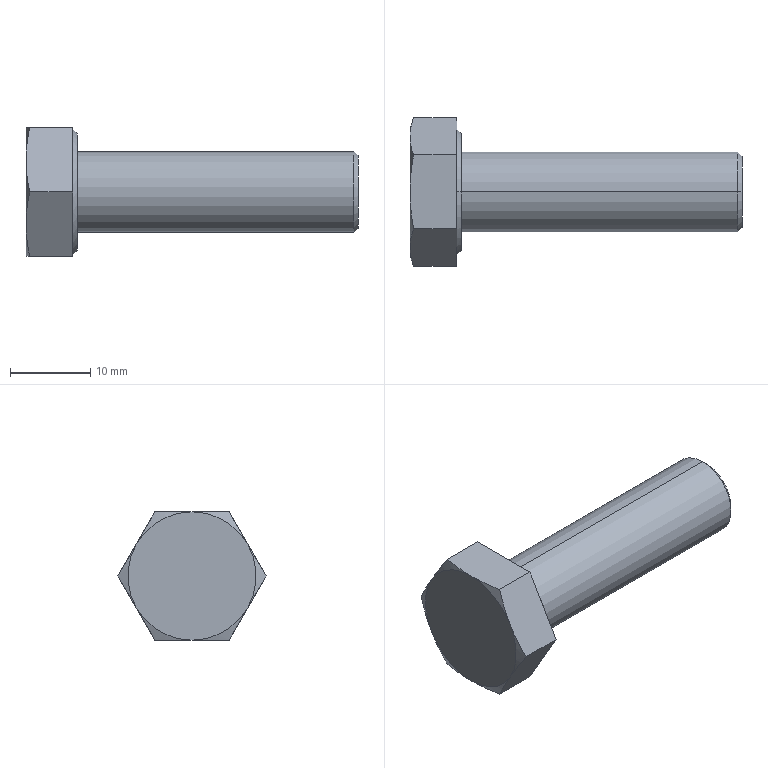Part | SolidWorks | features RevCut 3, Boss 1, Chamfer 1, Extrusion 1, Fillet 1, LPattern 1 | 1 solid | 22 faces | box 41.4 x 18.475 x 16 mm | volume 4135 mm3 | cone 10 | plane 10 | cylinder 2 | commonest cylinder face diameters 10 x2
STEP:
#1=CARTESIAN_POINT('',(41.4,0.,-4.5));
#2=VERTEX_POINT('',#1);
#3=CARTESIAN_POINT('',(41.4,0.,4.5));
#4=VERTEX_POINT('',#3);
#5=CARTESIAN_POINT('',(41.4,0.,0.));
#6=DIRECTION('',(1.,0.,0.));
#7=DIRECTION('',(0.,0.,-1.));
#8=AXIS2_PLACEMENT_3D('',#5,#6,#7);
#9=CIRCLE('',#8,4.5);
#10=EDGE_CURVE('',#2,#4,#9,.T.);
#11=ORIENTED_EDGE('',*,*,#10,.F.);
#12=CARTESIAN_POINT('',(40.9,0.,-5.));
#13=VERTEX_POINT('',#12);
#14=CARTESIAN_POINT('',(41.4,0.,-4.5));
#15=DIRECTION('',(-0.7071,0.,-0.7071));
#16=VECTOR('',#15,1000.);
#17=LINE('',#14,#16);
#18=EDGE_CURVE('',#2,#13,#17,.T.);
#19=ORIENTED_EDGE('',*,*,#18,.T.);
#20=CARTESIAN_POINT('',(40.9,0.,5.));
#21=VERTEX_POINT('',#20);
#22=CARTESIAN_POINT('',(40.9,0.,0.));
#23=DIRECTION('',(-1.,0.,0.));
#24=DIRECTION('',(0.,0.,-1.));
#25=AXIS2_PLACEMENT_3D('',#22,#23,#24);
#26=CIRCLE('',#25,5.);
#27=EDGE_CURVE('',#21,#13,#26,.T.);
#28=ORIENTED_EDGE('',*,*,#27,.F.);
#29=CARTESIAN_POINT('',(41.4,0.,4.5));
#30=DIRECTION('',(-0.7071,0.,0.7071));
#31=VECTOR('',#30,1000.);
#32=LINE('',#29,#31);
#33=EDGE_CURVE('',#4,#21,#32,.T.);
#34=ORIENTED_EDGE('',*,*,#33,.F.);
#35=EDGE_LOOP('',(#11,#19,#28,#34));
#36=FACE_OUTER_BOUND('',#35,.T.);
#37=CARTESIAN_POINT('',(41.4,0.,0.));
#38=DIRECTION('',(-1.,0.,0.));
#39=DIRECTION('',(0.,0.,1.));
#40=AXIS2_PLACEMENT_3D('',#37,#38,#39);
#41=CONICAL_SURFACE('',#40,4.5,0.7854);
#42=ADVANCED_FACE('',(#36),#41,.T.);
#43=ORIENTED_EDGE('',*,*,#27,.T.);
#44=CARTESIAN_POINT('',(6.4,0.,-5.));
#45=VERTEX_POINT('',#44);
#46=CARTESIAN_POINT('',(41.4,0.,-5.));
#47=DIRECTION('',(-1.,0.,0.));
#48=VECTOR('',#47,1000.);
#49=LINE('',#46,#48);
#50=EDGE_CURVE('',#13,#45,#49,.T.);
#51=ORIENTED_EDGE('',*,*,#50,.T.);
#52=CARTESIAN_POINT('',(6.4,0.,5.));
#53=VERTEX_POINT('',#52);
#54=CARTESIAN_POINT('',(6.4,0.,0.));
#55=DIRECTION('',(1.,0.,0.));
#56=DIRECTION('',(0.,0.,1.));
#57=AXIS2_PLACEMENT_3D('',#54,#55,#56);
#58=CIRCLE('',#57,5.);
#59=EDGE_CURVE('',#45,#53,#58,.T.);
#60=ORIENTED_EDGE('',*,*,#59,.T.);
#61=CARTESIAN_POINT('',(41.4,0.,5.));
#62=DIRECTION('',(-1.,0.,0.));
#63=VECTOR('',#62,1000.);
#64=LINE('',#61,#63);
#65=EDGE_CURVE('',#21,#53,#64,.T.);
#66=ORIENTED_EDGE('',*,*,#65,.F.);
#67=EDGE_LOOP('',(#43,#51,#60,#66));
#68=FACE_OUTER_BOUND('',#67,.T.);
#69=CARTESIAN_POINT('',(41.4,0.,0.));
#70=DIRECTION('',(-1.,0.,0.));
#71=DIRECTION('',(0.,0.,1.));
#72=AXIS2_PLACEMENT_3D('',#69,#70,#71);
#73=CYLINDRICAL_SURFACE('',#72,5.);
#74=ADVANCED_FACE('',(#68),#73,.T.);
#75=CARTESIAN_POINT('',(6.4,0.,7.235));
#76=VERTEX_POINT('',#75);
#77=CARTESIAN_POINT('',(6.4,0.,-7.235));
#78=VERTEX_POINT('',#77);
#79=CARTESIAN_POINT('',(6.4,0.,0.));
#80=DIRECTION('',(-1.,0.,0.));
#81=DIRECTION('',(0.,0.,1.));
#82=AXIS2_PLACEMENT_3D('',#79,#80,#81);
#83=CIRCLE('',#82,7.235);
#84=EDGE_CURVE('',#76,#78,#83,.T.);
#85=ORIENTED_EDGE('',*,*,#84,.T.);
#86=CARTESIAN_POINT('',(5.8,0.,-7.835));
#87=VERTEX_POINT('',#86);
#88=CARTESIAN_POINT('',(5.8,0.,-7.835));
#89=DIRECTION('',(-0.7071,0.,-0.7071));
#90=VECTOR('',#89,1000.);
#91=LINE('',#88,#90);
#92=EDGE_CURVE('',#78,#87,#91,.T.);
#93=ORIENTED_EDGE('',*,*,#92,.T.);
#94=CARTESIAN_POINT('',(5.8,0.,7.835));
#95=VERTEX_POINT('',#94);
#96=CARTESIAN_POINT('',(5.8,0.,0.));
#97=DIRECTION('',(-1.,0.,0.));
#98=DIRECTION('',(0.,0.,1.));
#99=AXIS2_PLACEMENT_3D('',#96,#97,#98);
#100=CIRCLE('',#99,7.835);
#101=EDGE_CURVE('',#95,#87,#100,.T.);
#102=ORIENTED_EDGE('',*,*,#101,.F.);
#103=CARTESIAN_POINT('',(5.8,0.,7.835));
#104=DIRECTION('',(-0.7071,0.,0.7071));
#105=VECTOR('',#104,1000.);
#106=LINE('',#103,#105);
#107=EDGE_CURVE('',#76,#95,#106,.T.);
#108=ORIENTED_EDGE('',*,*,#107,.F.);
#109=EDGE_LOOP('',(#85,#93,#102,#108));
#110=FACE_OUTER_BOUND('',#109,.T.);
#111=CARTESIAN_POINT('',(5.8,0.,0.));
#112=DIRECTION('',(-1.,0.,0.));
#113=DIRECTION('',(0.,0.,1.));
#114=AXIS2_PLACEMENT_3D('',#111,#112,#113);
#115=CONICAL_SURFACE('',#114,7.835,0.7854);
#116=ADVANCED_FACE('',(#110),#115,.T.);
#117=ORIENTED_EDGE('',*,*,#84,.F.);
#118=CARTESIAN_POINT('',(6.4,0.,0.));
#119=DIRECTION('',(-1.,0.,0.));
#120=DIRECTION('',(0.,0.,1.));
#121=AXIS2_PLACEMENT_3D('',#118,#119,#120);
#122=CIRCLE('',#121,7.235);
#123=EDGE_CURVE('',#78,#76,#122,.T.);
#124=ORIENTED_EDGE('',*,*,#123,.F.);
#125=EDGE_LOOP('',(#117,#124));
#126=FACE_OUTER_BOUND('',#125,.T.);
#127=CARTESIAN_POINT('',(6.4,0.,0.));
#128=DIRECTION('',(1.,0.,0.));
#129=DIRECTION('',(0.,0.,1.));
#130=AXIS2_PLACEMENT_3D('',#127,#128,#129);
#131=CIRCLE('',#130,5.);
#132=EDGE_CURVE('',#53,#45,#131,.T.);
#133=ORIENTED_EDGE('',*,*,#132,.F.);
#134=ORIENTED_EDGE('',*,*,#59,.F.);
#135=EDGE_LOOP('',(#133,#134));
#136=FACE_BOUND('',#135,.T.);
#137=CARTESIAN_POINT('',(6.4,0.,16.));
#138=DIRECTION('',(-1.,0.,0.));
#139=DIRECTION('',(0.,0.,1.));
#140=AXIS2_PLACEMENT_3D('',#137,#138,#139);
#141=PLANE('',#140);
#142=ADVANCED_FACE('',(#126,#136),#141,.F.);
#143=CARTESIAN_POINT('',(0.4505,-9.238,0.));
#144=VERTEX_POINT('',#143);
#145=CARTESIAN_POINT('',(0.,-6.928,4.));
#146=VERTEX_POINT('',#145);
#147=CARTESIAN_POINT('',(0.4505,-9.238,0.));
#148=CARTESIAN_POINT('',(0.3104,-8.853,0.6667));
#149=CARTESIAN_POINT('',(0.1966,-8.468,1.333));
#150=CARTESIAN_POINT('',(0.04119,-7.698,2.667));
#151=CARTESIAN_POINT('',(0.,-7.313,3.333));
#152=CARTESIAN_POINT('',(0.,-6.928,4.));
#153=B_SPLINE_CURVE_WITH_KNOTS('',3,(#147,#148,#149,#150,#151,#152),.UNSPECIFIED.,.F.,.F.,(4,2,4),(0.000000231,0.00231,0.004619),.UNSPECIFIED.);
#154=EDGE_CURVE('',#144,#146,#153,.T.);
#155=ORIENTED_EDGE('',*,*,#154,.F.);
#156=CARTESIAN_POINT('',(5.8,-9.238,0.));
#157=VERTEX_POINT('',#156);
#158=CARTESIAN_POINT('',(6.4,-9.238,0.));
#159=DIRECTION('',(-1.,0.,0.));
#160=VECTOR('',#159,1000.);
#161=LINE('',#158,#160);
#162=EDGE_CURVE('',#157,#144,#161,.T.);
#163=ORIENTED_EDGE('',*,*,#162,.F.);
#164=CARTESIAN_POINT('',(5.8,-4.619,8.));
#165=VERTEX_POINT('',#164);
#166=CARTESIAN_POINT('',(5.8,-4.619,8.));
#167=DIRECTION('',(0.,-0.5,-0.866));
#168=VECTOR('',#167,1000.);
#169=LINE('',#166,#168);
#170=EDGE_CURVE('',#165,#157,#169,.T.);
#171=ORIENTED_EDGE('',*,*,#170,.F.);
#172=CARTESIAN_POINT('',(0.4505,-4.619,8.));
#173=VERTEX_POINT('',#172);
#174=CARTESIAN_POINT('',(6.4,-4.619,8.));
#175=DIRECTION('',(-1.,0.,0.));
#176=VECTOR('',#175,1000.);
#177=LINE('',#174,#176);
#178=EDGE_CURVE('',#165,#173,#177,.T.);
#179=ORIENTED_EDGE('',*,*,#178,.T.);
#180=CARTESIAN_POINT('',(0.,-6.928,4.));
#181=CARTESIAN_POINT('',(0.,-6.543,4.667));
#182=CARTESIAN_POINT('',(0.04119,-6.158,5.333));
#183=CARTESIAN_POINT('',(0.1966,-5.389,6.667));
#184=CARTESIAN_POINT('',(0.3104,-5.004,7.333));
#185=CARTESIAN_POINT('',(0.4505,-4.619,8.));
#186=B_SPLINE_CURVE_WITH_KNOTS('',3,(#180,#181,#182,#183,#184,#185),.UNSPECIFIED.,.F.,.F.,(4,2,4),(0.004619,0.006928,0.009238),.UNSPECIFIED.);
#187=EDGE_CURVE('',#146,#173,#186,.T.);
#188=ORIENTED_EDGE('',*,*,#187,.F.);
#189=EDGE_LOOP('',(#155,#163,#171,#179,#188));
#190=FACE_OUTER_BOUND('',#189,.T.);
#191=CARTESIAN_POINT('',(6.4,-4.619,8.));
#192=DIRECTION('',(0.,0.866,-0.5));
#193=DIRECTION('',(0.,0.5,0.866));
#194=AXIS2_PLACEMENT_3D('',#191,#192,#193);
#195=PLANE('',#194);
#196=ADVANCED_FACE('',(#190),#195,.F.);
#197=CARTESIAN_POINT('',(0.4505,-4.619,-8.));
#198=VERTEX_POINT('',#197);
#199=CARTESIAN_POINT('',(0.,-6.928,-4.));
#200=VERTEX_POINT('',#199);
#201=CARTESIAN_POINT('',(0.4505,-4.619,-8.));
#202=CARTESIAN_POINT('',(0.3104,-5.004,-7.333));
#203=CARTESIAN_POINT('',(0.1966,-5.389,-6.667));
#204=CARTESIAN_POINT('',(0.04119,-6.158,-5.333));
#205=CARTESIAN_POINT('',(0.,-6.543,-4.667));
#206=CARTESIAN_POINT('',(0.,-6.928,-4.));
#207=B_SPLINE_CURVE_WITH_KNOTS('',3,(#201,#202,#203,#204,#205,#206),.UNSPECIFIED.,.F.,.F.,(4,2,4),(0.000000231,0.00231,0.004619),.UNSPECIFIED.);
#208=EDGE_CURVE('',#198,#200,#207,.T.);
#209=ORIENTED_EDGE('',*,*,#208,.F.);
#210=CARTESIAN_POINT('',(5.8,-4.619,-8.));
#211=VERTEX_POINT('',#210);
#212=CARTESIAN_POINT('',(6.4,-4.619,-8.));
#213=DIRECTION('',(-1.,0.,0.));
#214=VECTOR('',#213,1000.);
#215=LINE('',#212,#214);
#216=EDGE_CURVE('',#211,#198,#215,.T.);
#217=ORIENTED_EDGE('',*,*,#216,.F.);
#218=CARTESIAN_POINT('',(5.8,-9.238,0.));
#219=DIRECTION('',(0.,0.5,-0.866));
#220=VECTOR('',#219,1000.);
#221=LINE('',#218,#220);
#222=EDGE_CURVE('',#157,#211,#221,.T.);
#223=ORIENTED_EDGE('',*,*,#222,.F.);
#224=ORIENTED_EDGE('',*,*,#162,.T.);
#225=CARTESIAN_POINT('',(0.,-6.928,-4.));
#226=CARTESIAN_POINT('',(0.,-7.313,-3.333));
#227=CARTESIAN_POINT('',(0.04119,-7.698,-2.667));
#228=CARTESIAN_POINT('',(0.1966,-8.468,-1.333));
#229=CARTESIAN_POINT('',(0.3104,-8.853,-0.6667));
#230=CARTESIAN_POINT('',(0.4505,-9.238,0.));
#231=B_SPLINE_CURVE_WITH_KNOTS('',3,(#225,#226,#227,#228,#229,#230),.UNSPECIFIED.,.F.,.F.,(4,2,4),(0.004619,0.006928,0.009238),.UNSPECIFIED.);
#232=EDGE_CURVE('',#200,#144,#231,.T.);
#233=ORIENTED_EDGE('',*,*,#232,.F.);
#234=EDGE_LOOP('',(#209,#217,#223,#224,#233));
#235=FACE_OUTER_BOUND('',#234,.T.);
#236=CARTESIAN_POINT('',(6.4,-9.238,0.));
#237=DIRECTION('',(0.,0.866,0.5));
#238=DIRECTION('',(0.,-0.5,0.866));
#239=AXIS2_PLACEMENT_3D('',#236,#237,#238);
#240=PLANE('',#239);
#241=ADVANCED_FACE('',(#235),#240,.F.);
#242=CARTESIAN_POINT('',(0.4505,4.619,-8.));
#243=VERTEX_POINT('',#242);
#244=CARTESIAN_POINT('',(0.,0.,-8.));
#245=VERTEX_POINT('',#244);
#246=CARTESIAN_POINT('',(0.4505,4.619,-8.));
#247=CARTESIAN_POINT('',(0.3107,3.851,-8.));
#248=CARTESIAN_POINT('',(0.1969,3.081,-8.));
#249=CARTESIAN_POINT('',(0.04135,1.542,-8.));
#250=CARTESIAN_POINT('',(0.,0.7714,-8.));
#251=CARTESIAN_POINT('',(0.,0.,-8.));
#252=B_SPLINE_CURVE_WITH_KNOTS('',3,(#246,#247,#248,#249,#250,#251),.UNSPECIFIED.,.F.,.F.,(4,2,4),(0.01666,0.01898,0.02131),.UNSPECIFIED.);
#253=EDGE_CURVE('',#243,#245,#252,.T.);
#254=ORIENTED_EDGE('',*,*,#253,.F.);
#255=CARTESIAN_POINT('',(5.8,4.619,-8.));
#256=VERTEX_POINT('',#255);
#257=CARTESIAN_POINT('',(6.4,4.619,-8.));
#258=DIRECTION('',(-1.,0.,0.));
#259=VECTOR('',#258,1000.);
#260=LINE('',#257,#259);
#261=EDGE_CURVE('',#256,#243,#260,.T.);
#262=ORIENTED_EDGE('',*,*,#261,.F.);
#263=CARTESIAN_POINT('',(5.8,-4.619,-8.));
#264=DIRECTION('',(0.,1.,0.));
#265=VECTOR('',#264,1000.);
#266=LINE('',#263,#265);
#267=EDGE_CURVE('',#211,#256,#266,.T.);
#268=ORIENTED_EDGE('',*,*,#267,.F.);
#269=ORIENTED_EDGE('',*,*,#216,.T.);
#270=CARTESIAN_POINT('',(0.,0.,-8.));
#271=CARTESIAN_POINT('',(0.,-0.7692,-8.));
#272=CARTESIAN_POINT('',(0.04113,-1.539,-8.));
#273=CARTESIAN_POINT('',(0.1968,-3.081,-8.));
#274=CARTESIAN_POINT('',(0.3113,-3.854,-8.));
#275=CARTESIAN_POINT('',(0.4505,-4.619,-8.));
#276=B_SPLINE_CURVE_WITH_KNOTS('',3,(#270,#271,#272,#273,#274,#275),.UNSPECIFIED.,.F.,.F.,(4,2,4),(0.02131,0.02363,0.02596),.UNSPECIFIED.);
#277=EDGE_CURVE('',#245,#198,#276,.T.);
#278=ORIENTED_EDGE('',*,*,#277,.F.);
#279=EDGE_LOOP('',(#254,#262,#268,#269,#278));
#280=FACE_OUTER_BOUND('',#279,.T.);
#281=CARTESIAN_POINT('',(6.4,-4.619,-8.));
#282=DIRECTION('',(0.,0.,1.));
#283=DIRECTION('',(0.,-1.,0.));
#284=AXIS2_PLACEMENT_3D('',#281,#282,#283);
#285=PLANE('',#284);
#286=ADVANCED_FACE('',(#280),#285,.F.);
#287=CARTESIAN_POINT('',(0.4505,9.238,0.));
#288=VERTEX_POINT('',#287);
#289=CARTESIAN_POINT('',(0.,6.928,-4.));
#290=VERTEX_POINT('',#289);
#291=CARTESIAN_POINT('',(0.4505,9.238,0.));
#292=CARTESIAN_POINT('',(0.3104,8.853,-0.6667));
#293=CARTESIAN_POINT('',(0.1966,8.468,-1.333));
#294=CARTESIAN_POINT('',(0.04119,7.698,-2.667));
#295=CARTESIAN_POINT('',(0.,7.313,-3.333));
#296=CARTESIAN_POINT('',(0.,6.928,-4.));
#297=B_SPLINE_CURVE_WITH_KNOTS('',3,(#291,#292,#293,#294,#295,#296),.UNSPECIFIED.,.F.,.F.,(4,2,4),(0.000000231,0.00231,0.004619),.UNSPECIFIED.);
#298=EDGE_CURVE('',#288,#290,#297,.T.);
#299=ORIENTED_EDGE('',*,*,#298,.F.);
#300=CARTESIAN_POINT('',(5.8,9.238,0.));
#301=VERTEX_POINT('',#300);
#302=CARTESIAN_POINT('',(6.4,9.238,0.));
#303=DIRECTION('',(-1.,0.,0.));
#304=VECTOR('',#303,1000.);
#305=LINE('',#302,#304);
#306=EDGE_CURVE('',#301,#288,#305,.T.);
#307=ORIENTED_EDGE('',*,*,#306,.F.);
#308=CARTESIAN_POINT('',(5.8,4.619,-8.));
#309=DIRECTION('',(0.,0.5,0.866));
#310=VECTOR('',#309,1000.);
#311=LINE('',#308,#310);
#312=EDGE_CURVE('',#256,#301,#311,.T.);
#313=ORIENTED_EDGE('',*,*,#312,.F.);
#314=ORIENTED_EDGE('',*,*,#261,.T.);
#315=CARTESIAN_POINT('',(0.,6.928,-4.));
#316=CARTESIAN_POINT('',(0.,6.543,-4.667));
#317=CARTESIAN_POINT('',(0.04119,6.158,-5.333));
#318=CARTESIAN_POINT('',(0.1966,5.389,-6.667));
#319=CARTESIAN_POINT('',(0.3104,5.004,-7.333));
#320=CARTESIAN_POINT('',(0.4505,4.619,-8.));
#321=B_SPLINE_CURVE_WITH_KNOTS('',3,(#315,#316,#317,#318,#319,#320),.UNSPECIFIED.,.F.,.F.,(4,2,4),(0.004619,0.006928,0.009238),.UNSPECIFIED.);
#322=EDGE_CURVE('',#290,#243,#321,.T.);
#323=ORIENTED_EDGE('',*,*,#322,.F.);
#324=EDGE_LOOP('',(#299,#307,#313,#314,#323));
#325=FACE_OUTER_BOUND('',#324,.T.);
#326=CARTESIAN_POINT('',(6.4,4.619,-8.));
#327=DIRECTION('',(0.,-0.866,0.5));
#328=DIRECTION('',(0.,-0.5,-0.866));
#329=AXIS2_PLACEMENT_3D('',#326,#327,#328);
#330=PLANE('',#329);
#331=ADVANCED_FACE('',(#325),#330,.F.);
#332=CARTESIAN_POINT('',(0.4505,4.619,8.));
#333=VERTEX_POINT('',#332);
#334=CARTESIAN_POINT('',(0.,6.928,4.));
#335=VERTEX_POINT('',#334);
#336=CARTESIAN_POINT('',(0.4505,4.619,8.));
#337=CARTESIAN_POINT('',(0.3104,5.004,7.333));
#338=CARTESIAN_POINT('',(0.1966,5.389,6.667));
#339=CARTESIAN_POINT('',(0.04119,6.158,5.333));
#340=CARTESIAN_POINT('',(0.,6.543,4.667));
#341=CARTESIAN_POINT('',(0.,6.928,4.));
#342=B_SPLINE_CURVE_WITH_KNOTS('',3,(#336,#337,#338,#339,#340,#341),.UNSPECIFIED.,.F.,.F.,(4,2,4),(0.000000231,0.00231,0.004619),.UNSPECIFIED.);
#343=EDGE_CURVE('',#333,#335,#342,.T.);
#344=ORIENTED_EDGE('',*,*,#343,.F.);
#345=CARTESIAN_POINT('',(5.8,4.619,8.));
#346=VERTEX_POINT('',#345);
#347=CARTESIAN_POINT('',(6.4,4.619,8.));
#348=DIRECTION('',(-1.,0.,0.));
#349=VECTOR('',#348,1000.);
#350=LINE('',#347,#349);
#351=EDGE_CURVE('',#346,#333,#350,.T.);
#352=ORIENTED_EDGE('',*,*,#351,.F.);
#353=CARTESIAN_POINT('',(5.8,9.238,0.));
#354=DIRECTION('',(0.,-0.5,0.866));
#355=VECTOR('',#354,1000.);
#356=LINE('',#353,#355);
#357=EDGE_CURVE('',#301,#346,#356,.T.);
#358=ORIENTED_EDGE('',*,*,#357,.F.);
#359=ORIENTED_EDGE('',*,*,#306,.T.);
#360=CARTESIAN_POINT('',(0.,6.928,4.));
#361=CARTESIAN_POINT('',(0.,7.313,3.333));
#362=CARTESIAN_POINT('',(0.04119,7.698,2.667));
#363=CARTESIAN_POINT('',(0.1966,8.468,1.333));
#364=CARTESIAN_POINT('',(0.3104,8.853,0.6667));
#365=CARTESIAN_POINT('',(0.4505,9.238,0.));
#366=B_SPLINE_CURVE_WITH_KNOTS('',3,(#360,#361,#362,#363,#364,#365),.UNSPECIFIED.,.F.,.F.,(4,2,4),(0.004619,0.006928,0.009238),.UNSPECIFIED.);
#367=EDGE_CURVE('',#335,#288,#366,.T.);
#368=ORIENTED_EDGE('',*,*,#367,.F.);
#369=EDGE_LOOP('',(#344,#352,#358,#359,#368));
#370=FACE_OUTER_BOUND('',#369,.T.);
#371=CARTESIAN_POINT('',(6.4,9.238,0.));
#372=DIRECTION('',(0.,-0.866,-0.5));
#373=DIRECTION('',(0.,0.5,-0.866));
#374=AXIS2_PLACEMENT_3D('',#371,#372,#373);
#375=PLANE('',#374);
#376=ADVANCED_FACE('',(#370),#375,.F.);
#377=CARTESIAN_POINT('',(0.,0.,8.));
#378=VERTEX_POINT('',#377);
#379=CARTESIAN_POINT('',(0.4505,-4.619,8.));
#380=CARTESIAN_POINT('',(0.3113,-3.854,8.));
#381=CARTESIAN_POINT('',(0.1968,-3.081,8.));
#382=CARTESIAN_POINT('',(0.04113,-1.539,8.));
#383=CARTESIAN_POINT('',(0.,-0.7692,8.));
#384=CARTESIAN_POINT('',(0.,0.,8.));
#385=B_SPLINE_CURVE_WITH_KNOTS('',3,(#379,#380,#381,#382,#383,#384),.UNSPECIFIED.,.F.,.F.,(4,2,4),(0.007857,0.01018,0.01251),.UNSPECIFIED.);
#386=EDGE_CURVE('',#173,#378,#385,.T.);
#387=ORIENTED_EDGE('',*,*,#386,.F.);
#388=ORIENTED_EDGE('',*,*,#178,.F.);
#389=CARTESIAN_POINT('',(5.8,4.619,8.));
#390=DIRECTION('',(0.,-1.,0.));
#391=VECTOR('',#390,1000.);
#392=LINE('',#389,#391);
#393=EDGE_CURVE('',#346,#165,#392,.T.);
#394=ORIENTED_EDGE('',*,*,#393,.F.);
#395=ORIENTED_EDGE('',*,*,#351,.T.);
#396=CARTESIAN_POINT('',(0.,0.,8.));
#397=CARTESIAN_POINT('',(0.,0.7714,8.));
#398=CARTESIAN_POINT('',(0.04135,1.542,8.));
#399=CARTESIAN_POINT('',(0.1969,3.081,8.));
#400=CARTESIAN_POINT('',(0.3107,3.851,8.));
#401=CARTESIAN_POINT('',(0.4505,4.619,8.));
#402=B_SPLINE_CURVE_WITH_KNOTS('',3,(#396,#397,#398,#399,#400,#401),.UNSPECIFIED.,.F.,.F.,(4,2,4),(0.01251,0.01485,0.01718),.UNSPECIFIED.);
#403=EDGE_CURVE('',#378,#333,#402,.T.);
#404=ORIENTED_EDGE('',*,*,#403,.F.);
#405=EDGE_LOOP('',(#387,#388,#394,#395,#404));
#406=FACE_OUTER_BOUND('',#405,.T.);
#407=CARTESIAN_POINT('',(6.4,4.619,8.));
#408=DIRECTION('',(0.,0.,-1.));
#409=DIRECTION('',(-1.,0.,0.));
#410=AXIS2_PLACEMENT_3D('',#407,#408,#409);
#411=PLANE('',#410);
#412=ADVANCED_FACE('',(#406),#411,.F.);
#413=ORIENTED_EDGE('',*,*,#101,.T.);
#414=CARTESIAN_POINT('',(5.8,0.,0.));
#415=DIRECTION('',(-1.,0.,0.));
#416=DIRECTION('',(0.,0.,1.));
#417=AXIS2_PLACEMENT_3D('',#414,#415,#416);
#418=CIRCLE('',#417,7.835);
#419=EDGE_CURVE('',#87,#95,#418,.T.);
#420=ORIENTED_EDGE('',*,*,#419,.T.);
#421=EDGE_LOOP('',(#413,#420));
#422=FACE_BOUND('',#421,.T.);
#423=ORIENTED_EDGE('',*,*,#170,.T.);
#424=ORIENTED_EDGE('',*,*,#222,.T.);
#425=ORIENTED_EDGE('',*,*,#267,.T.);
#426=ORIENTED_EDGE('',*,*,#312,.T.);
#427=ORIENTED_EDGE('',*,*,#357,.T.);
#428=ORIENTED_EDGE('',*,*,#393,.T.);
#429=EDGE_LOOP('',(#423,#424,#425,#426,#427,#428));
#430=FACE_OUTER_BOUND('',#429,.T.);
#431=CARTESIAN_POINT('',(5.8,7.835,0.));
#432=DIRECTION('',(1.,0.,0.));
#433=DIRECTION('',(0.,0.,-1.));
#434=AXIS2_PLACEMENT_3D('',#431,#432,#433);
#435=PLANE('',#434);
#436=ADVANCED_FACE('',(#422,#430),#435,.T.);
#437=ORIENTED_EDGE('',*,*,#92,.F.);
#438=ORIENTED_EDGE('',*,*,#123,.T.);
#439=ORIENTED_EDGE('',*,*,#107,.T.);
#440=ORIENTED_EDGE('',*,*,#419,.F.);
#441=EDGE_LOOP('',(#437,#438,#439,#440));
#442=FACE_OUTER_BOUND('',#441,.T.);
#443=CARTESIAN_POINT('',(5.8,0.,0.));
#444=DIRECTION('',(-1.,0.,0.));
#445=DIRECTION('',(0.,0.,1.));
#446=AXIS2_PLACEMENT_3D('',#443,#444,#445);
#447=CONICAL_SURFACE('',#446,7.835,0.7854);
#448=ADVANCED_FACE('',(#442),#447,.T.);
#449=ORIENTED_EDGE('',*,*,#187,.T.);
#450=ORIENTED_EDGE('',*,*,#386,.T.);
#451=CARTESIAN_POINT('',(0.,0.,0.));
#452=DIRECTION('',(-1.,0.,0.));
#453=DIRECTION('',(0.,0.,1.));
#454=AXIS2_PLACEMENT_3D('',#451,#452,#453);
#455=CIRCLE('',#454,8.);
#456=EDGE_CURVE('',#146,#378,#455,.T.);
#457=ORIENTED_EDGE('',*,*,#456,.F.);
#458=EDGE_LOOP('',(#449,#450,#457));
#459=FACE_OUTER_BOUND('',#458,.T.);
#460=CARTESIAN_POINT('',(0.,0.,0.));
#461=DIRECTION('',(1.,0.,0.));
#462=DIRECTION('',(0.,0.,-1.));
#463=AXIS2_PLACEMENT_3D('',#460,#461,#462);
#464=CONICAL_SURFACE('',#463,8.,1.222);
#465=ADVANCED_FACE('',(#459),#464,.T.);
#466=ORIENTED_EDGE('',*,*,#232,.T.);
#467=ORIENTED_EDGE('',*,*,#154,.T.);
#468=CARTESIAN_POINT('',(0.,0.,0.));
#469=DIRECTION('',(-1.,0.,0.));
#470=DIRECTION('',(0.,0.,1.));
#471=AXIS2_PLACEMENT_3D('',#468,#469,#470);
#472=CIRCLE('',#471,8.);
#473=EDGE_CURVE('',#200,#146,#472,.T.);
#474=ORIENTED_EDGE('',*,*,#473,.F.);
#475=EDGE_LOOP('',(#466,#467,#474));
#476=FACE_OUTER_BOUND('',#475,.T.);
#477=CARTESIAN_POINT('',(0.,0.,0.));
#478=DIRECTION('',(1.,0.,0.));
#479=DIRECTION('',(0.,0.,-1.));
#480=AXIS2_PLACEMENT_3D('',#477,#478,#479);
#481=CONICAL_SURFACE('',#480,8.,1.222);
#482=ADVANCED_FACE('',(#476),#481,.T.);
#483=ORIENTED_EDGE('',*,*,#277,.T.);
#484=ORIENTED_EDGE('',*,*,#208,.T.);
#485=CARTESIAN_POINT('',(0.,0.,0.));
#486=DIRECTION('',(-1.,0.,0.));
#487=DIRECTION('',(0.,0.,1.));
#488=AXIS2_PLACEMENT_3D('',#485,#486,#487);
#489=CIRCLE('',#488,8.);
#490=EDGE_CURVE('',#245,#200,#489,.T.);
#491=ORIENTED_EDGE('',*,*,#490,.F.);
#492=EDGE_LOOP('',(#483,#484,#491));
#493=FACE_OUTER_BOUND('',#492,.T.);
#494=CARTESIAN_POINT('',(0.,0.,0.));
#495=DIRECTION('',(1.,0.,0.));
#496=DIRECTION('',(0.,0.,-1.));
#497=AXIS2_PLACEMENT_3D('',#494,#495,#496);
#498=CONICAL_SURFACE('',#497,8.,1.222);
#499=ADVANCED_FACE('',(#493),#498,.T.);
#500=ORIENTED_EDGE('',*,*,#253,.T.);
#501=CARTESIAN_POINT('',(0.,0.,0.));
#502=DIRECTION('',(-1.,0.,0.));
#503=DIRECTION('',(0.,0.,1.));
#504=AXIS2_PLACEMENT_3D('',#501,#502,#503);
#505=CIRCLE('',#504,8.);
#506=EDGE_CURVE('',#290,#245,#505,.T.);
#507=ORIENTED_EDGE('',*,*,#506,.F.);
#508=ORIENTED_EDGE('',*,*,#322,.T.);
#509=EDGE_LOOP('',(#500,#507,#508));
#510=FACE_OUTER_BOUND('',#509,.T.);
#511=CARTESIAN_POINT('',(0.,0.,0.));
#512=DIRECTION('',(1.,0.,0.));
#513=DIRECTION('',(0.,0.,-1.));
#514=AXIS2_PLACEMENT_3D('',#511,#512,#513);
#515=CONICAL_SURFACE('',#514,8.,1.222);
#516=ADVANCED_FACE('',(#510),#515,.T.);
#517=ORIENTED_EDGE('',*,*,#298,.T.);
#518=CARTESIAN_POINT('',(0.,0.,0.));
#519=DIRECTION('',(-1.,0.,0.));
#520=DIRECTION('',(0.,0.,1.));
#521=AXIS2_PLACEMENT_3D('',#518,#519,#520);
#522=CIRCLE('',#521,8.);
#523=EDGE_CURVE('',#335,#290,#522,.T.);
#524=ORIENTED_EDGE('',*,*,#523,.F.);
#525=ORIENTED_EDGE('',*,*,#367,.T.);
#526=EDGE_LOOP('',(#517,#524,#525));
#527=FACE_OUTER_BOUND('',#526,.T.);
#528=CARTESIAN_POINT('',(0.,0.,0.));
#529=DIRECTION('',(1.,0.,0.));
#530=DIRECTION('',(0.,0.,-1.));
#531=AXIS2_PLACEMENT_3D('',#528,#529,#530);
#532=CONICAL_SURFACE('',#531,8.,1.222);
#533=ADVANCED_FACE('',(#527),#532,.T.);
#534=ORIENTED_EDGE('',*,*,#343,.T.);
#535=CARTESIAN_POINT('',(0.,0.,0.));
#536=DIRECTION('',(-1.,0.,0.));
#537=DIRECTION('',(0.,0.,1.));
#538=AXIS2_PLACEMENT_3D('',#535,#536,#537);
#539=CIRCLE('',#538,8.);
#540=EDGE_CURVE('',#378,#335,#539,.T.);
#541=ORIENTED_EDGE('',*,*,#540,.F.);
#542=ORIENTED_EDGE('',*,*,#403,.T.);
#543=EDGE_LOOP('',(#534,#541,#542));
#544=FACE_OUTER_BOUND('',#543,.T.);
#545=CARTESIAN_POINT('',(0.,0.,0.));
#546=DIRECTION('',(1.,0.,0.));
#547=DIRECTION('',(0.,0.,-1.));
#548=AXIS2_PLACEMENT_3D('',#545,#546,#547);
#549=CONICAL_SURFACE('',#548,8.,1.222);
#550=ADVANCED_FACE('',(#544),#549,.T.);
#551=ORIENTED_EDGE('',*,*,#456,.T.);
#552=ORIENTED_EDGE('',*,*,#540,.T.);
#553=ORIENTED_EDGE('',*,*,#523,.T.);
#554=ORIENTED_EDGE('',*,*,#506,.T.);
#555=ORIENTED_EDGE('',*,*,#490,.T.);
#556=ORIENTED_EDGE('',*,*,#473,.T.);
#557=EDGE_LOOP('',(#551,#552,#553,#554,#555,#556));
#558=FACE_OUTER_BOUND('',#557,.T.);
#559=CARTESIAN_POINT('',(0.,0.,16.));
#560=DIRECTION('',(-1.,0.,0.));
#561=DIRECTION('',(0.,0.,1.));
#562=AXIS2_PLACEMENT_3D('',#559,#560,#561);
#563=PLANE('',#562);
#564=ADVANCED_FACE('',(#558),#563,.T.);
#565=ORIENTED_EDGE('',*,*,#50,.F.);
#566=CARTESIAN_POINT('',(40.9,0.,0.));
#567=DIRECTION('',(-1.,0.,0.));
#568=DIRECTION('',(0.,0.,-1.));
#569=AXIS2_PLACEMENT_3D('',#566,#567,#568);
#570=CIRCLE('',#569,5.);
#571=EDGE_CURVE('',#13,#21,#570,.T.);
#572=ORIENTED_EDGE('',*,*,#571,.T.);
#573=ORIENTED_EDGE('',*,*,#65,.T.);
#574=ORIENTED_EDGE('',*,*,#132,.T.);
#575=EDGE_LOOP('',(#565,#572,#573,#574));
#576=FACE_OUTER_BOUND('',#575,.T.);
#577=CARTESIAN_POINT('',(41.4,0.,0.));
#578=DIRECTION('',(-1.,0.,0.));
#579=DIRECTION('',(0.,0.,1.));
#580=AXIS2_PLACEMENT_3D('',#577,#578,#579);
#581=CYLINDRICAL_SURFACE('',#580,5.);
#582=ADVANCED_FACE('',(#576),#581,.T.);
#583=CARTESIAN_POINT('',(41.4,0.,0.));
#584=DIRECTION('',(1.,0.,0.));
#585=DIRECTION('',(0.,0.,-1.));
#586=AXIS2_PLACEMENT_3D('',#583,#584,#585);
#587=CIRCLE('',#586,4.5);
#588=EDGE_CURVE('',#4,#2,#587,.T.);
#589=ORIENTED_EDGE('',*,*,#588,.T.);
#590=ORIENTED_EDGE('',*,*,#10,.T.);
#591=EDGE_LOOP('',(#589,#590));
#592=FACE_OUTER_BOUND('',#591,.T.);
#593=CARTESIAN_POINT('',(41.4,0.,0.));
#594=DIRECTION('',(1.,0.,0.));
#595=DIRECTION('',(0.,0.,-1.));
#596=AXIS2_PLACEMENT_3D('',#593,#594,#595);
#597=PLANE('',#596);
#598=ADVANCED_FACE('',(#592),#597,.T.);
#599=ORIENTED_EDGE('',*,*,#18,.F.);
#600=ORIENTED_EDGE('',*,*,#588,.F.);
#601=ORIENTED_EDGE('',*,*,#33,.T.);
#602=ORIENTED_EDGE('',*,*,#571,.F.);
#603=EDGE_LOOP('',(#599,#600,#601,#602));
#604=FACE_OUTER_BOUND('',#603,.T.);
#605=CARTESIAN_POINT('',(41.4,0.,0.));
#606=DIRECTION('',(-1.,0.,0.));
#607=DIRECTION('',(0.,0.,1.));
#608=AXIS2_PLACEMENT_3D('',#605,#606,#607);
#609=CONICAL_SURFACE('',#608,4.5,0.7854);
#610=ADVANCED_FACE('',(#604),#609,.T.);
#611=CLOSED_SHELL('',(#42,#74,#116,#142,#196,#241,#286,#331,#376,#412,#436,#448,#465,#482,#499,#516,#533,#550,#564,#582,#598,#610));
#612=MANIFOLD_SOLID_BREP('',#611);
#613=CARTESIAN_POINT('',(0.,0.,0.));
#614=DIRECTION('',(0.,0.,1.));
#615=DIRECTION('',(1.,0.,0.));
#616=AXIS2_PLACEMENT_3D('',#613,#614,#615);
#617=(LENGTH_UNIT()NAMED_UNIT(*)SI_UNIT(.MILLI.,.METRE.));
#618=UNCERTAINTY_MEASURE_WITH_UNIT(LENGTH_MEASURE(0.00001),#617,'','');
#619=(NAMED_UNIT(*)PLANE_ANGLE_UNIT()SI_UNIT($,.RADIAN.));
#620=(NAMED_UNIT(*)SI_UNIT($,.STERADIAN.)SOLID_ANGLE_UNIT());
#621=(GEOMETRIC_REPRESENTATION_CONTEXT(3)GLOBAL_UNCERTAINTY_ASSIGNED_CONTEXT((#618))GLOBAL_UNIT_ASSIGNED_CONTEXT((#617,#619,#620))REPRESENTATION_CONTEXT('',''));
#622=ADVANCED_BREP_SHAPE_REPRESENTATION('',(#612,#616),#621);